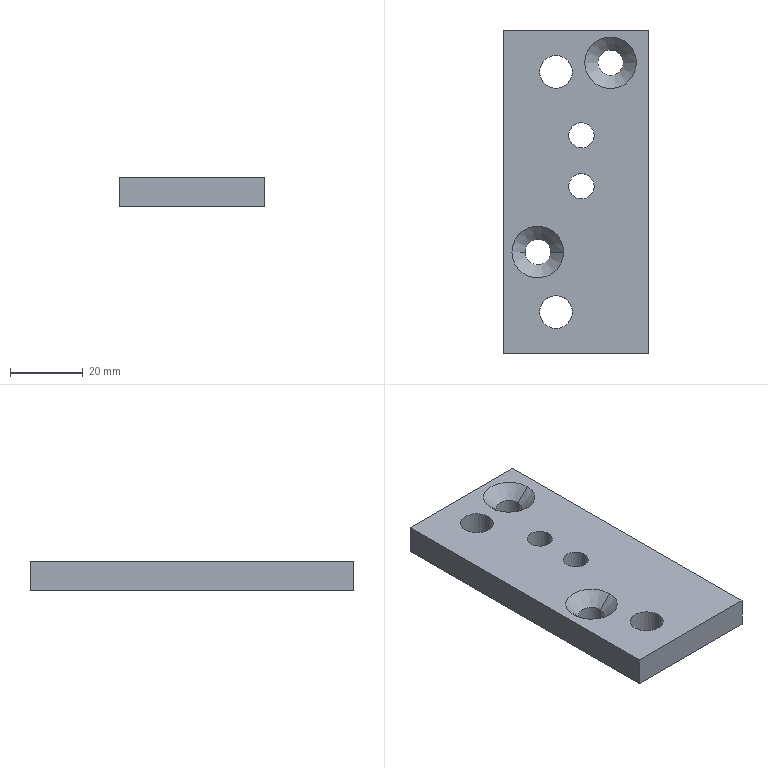Part | 1 solid | 22 faces | box 40 x 89 x 8 mm | volume 25848 mm3 | cylinder 12 | plane 6 | cone 4 | commonest cylinder face diameters 7 x8 9 x4